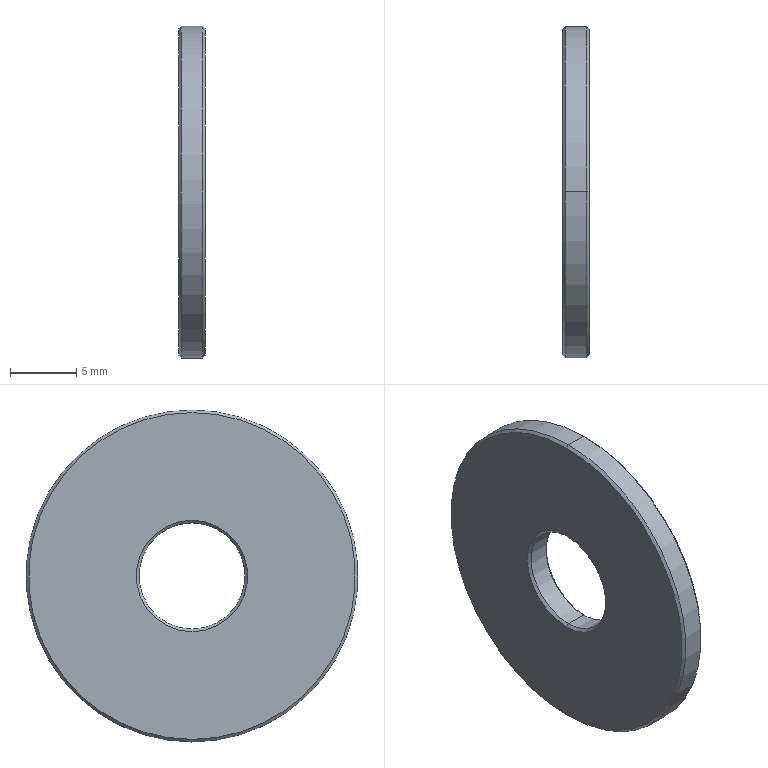Part | STEP file | WSSS25-8-2 | 1 solid | 14 faces | box 2 x 25 x 25 mm | volume 877.07 mm3 | cone 8 | cylinder 4 | plane 2 | commonest cylinder face diameters 8 x2 25 x2
STEP:
#1=CARTESIAN_POINT('',(2.,0.,-12.3));
#2=VERTEX_POINT('',#1);
#3=CARTESIAN_POINT('',(2.,0.,12.3));
#4=VERTEX_POINT('',#3);
#5=CARTESIAN_POINT('',(2.,0.,0.));
#6=DIRECTION('',(1.,0.,0.));
#7=DIRECTION('',(0.,0.,1.));
#8=AXIS2_PLACEMENT_3D('',#5,#6,#7);
#9=CIRCLE('',#8,12.3);
#10=EDGE_CURVE('',#2,#4,#9,.T.);
#11=ORIENTED_EDGE('',*,*,#10,.F.);
#12=CARTESIAN_POINT('',(1.8,0.,-12.5));
#13=VERTEX_POINT('',#12);
#14=CARTESIAN_POINT('',(1.8,0.,-12.5));
#15=DIRECTION('',(-0.7071,0.,-0.7071));
#16=VECTOR('',#15,1000.);
#17=LINE('',#14,#16);
#18=EDGE_CURVE('',#2,#13,#17,.T.);
#19=ORIENTED_EDGE('',*,*,#18,.T.);
#20=CARTESIAN_POINT('',(1.8,0.,12.5));
#21=VERTEX_POINT('',#20);
#22=CARTESIAN_POINT('',(1.8,0.,0.));
#23=DIRECTION('',(-1.,0.,0.));
#24=DIRECTION('',(0.,0.,1.));
#25=AXIS2_PLACEMENT_3D('',#22,#23,#24);
#26=CIRCLE('',#25,12.5);
#27=EDGE_CURVE('',#21,#13,#26,.T.);
#28=ORIENTED_EDGE('',*,*,#27,.F.);
#29=CARTESIAN_POINT('',(1.8,0.,12.5));
#30=DIRECTION('',(-0.7071,0.,0.7071));
#31=VECTOR('',#30,1000.);
#32=LINE('',#29,#31);
#33=EDGE_CURVE('',#4,#21,#32,.T.);
#34=ORIENTED_EDGE('',*,*,#33,.F.);
#35=EDGE_LOOP('',(#11,#19,#28,#34));
#36=FACE_OUTER_BOUND('',#35,.T.);
#37=CARTESIAN_POINT('',(1.8,0.,0.));
#38=DIRECTION('',(-1.,0.,0.));
#39=DIRECTION('',(0.,0.,1.));
#40=AXIS2_PLACEMENT_3D('',#37,#38,#39);
#41=CONICAL_SURFACE('',#40,12.5,0.7854);
#42=ADVANCED_FACE('',(#36),#41,.T.);
#43=CARTESIAN_POINT('',(1.8,0.,4.));
#44=VERTEX_POINT('',#43);
#45=CARTESIAN_POINT('',(1.8,0.,-4.));
#46=VERTEX_POINT('',#45);
#47=CARTESIAN_POINT('',(1.8,0.,0.));
#48=DIRECTION('',(1.,0.,0.));
#49=DIRECTION('',(0.,0.,1.));
#50=AXIS2_PLACEMENT_3D('',#47,#48,#49);
#51=CIRCLE('',#50,4.);
#52=EDGE_CURVE('',#44,#46,#51,.T.);
#53=ORIENTED_EDGE('',*,*,#52,.F.);
#54=CARTESIAN_POINT('',(2.,0.,4.2));
#55=VERTEX_POINT('',#54);
#56=CARTESIAN_POINT('',(2.,0.,4.2));
#57=DIRECTION('',(0.7071,0.,0.7071));
#58=VECTOR('',#57,1000.);
#59=LINE('',#56,#58);
#60=EDGE_CURVE('',#44,#55,#59,.T.);
#61=ORIENTED_EDGE('',*,*,#60,.T.);
#62=CARTESIAN_POINT('',(2.,0.,-4.2));
#63=VERTEX_POINT('',#62);
#64=CARTESIAN_POINT('',(2.,0.,0.));
#65=DIRECTION('',(-1.,0.,0.));
#66=DIRECTION('',(0.,0.,1.));
#67=AXIS2_PLACEMENT_3D('',#64,#65,#66);
#68=CIRCLE('',#67,4.2);
#69=EDGE_CURVE('',#63,#55,#68,.T.);
#70=ORIENTED_EDGE('',*,*,#69,.F.);
#71=CARTESIAN_POINT('',(2.,0.,-4.2));
#72=DIRECTION('',(0.7071,0.,-0.7071));
#73=VECTOR('',#72,1000.);
#74=LINE('',#71,#73);
#75=EDGE_CURVE('',#46,#63,#74,.T.);
#76=ORIENTED_EDGE('',*,*,#75,.F.);
#77=EDGE_LOOP('',(#53,#61,#70,#76));
#78=FACE_OUTER_BOUND('',#77,.T.);
#79=CARTESIAN_POINT('',(2.,0.,0.));
#80=DIRECTION('',(1.,0.,0.));
#81=DIRECTION('',(0.,0.,-1.));
#82=AXIS2_PLACEMENT_3D('',#79,#80,#81);
#83=CONICAL_SURFACE('',#82,4.2,0.7854);
#84=ADVANCED_FACE('',(#78),#83,.F.);
#85=CARTESIAN_POINT('',(0.,0.,12.3));
#86=VERTEX_POINT('',#85);
#87=CARTESIAN_POINT('',(0.,0.,-12.3));
#88=VERTEX_POINT('',#87);
#89=CARTESIAN_POINT('',(0.,0.,0.));
#90=DIRECTION('',(-1.,0.,0.));
#91=DIRECTION('',(0.,0.,-1.));
#92=AXIS2_PLACEMENT_3D('',#89,#90,#91);
#93=CIRCLE('',#92,12.3);
#94=EDGE_CURVE('',#86,#88,#93,.T.);
#95=ORIENTED_EDGE('',*,*,#94,.F.);
#96=CARTESIAN_POINT('',(0.2,0.,12.5));
#97=VERTEX_POINT('',#96);
#98=CARTESIAN_POINT('',(0.,0.,12.3));
#99=DIRECTION('',(0.7071,0.,0.7071));
#100=VECTOR('',#99,1000.);
#101=LINE('',#98,#100);
#102=EDGE_CURVE('',#86,#97,#101,.T.);
#103=ORIENTED_EDGE('',*,*,#102,.T.);
#104=CARTESIAN_POINT('',(0.2,0.,-12.5));
#105=VERTEX_POINT('',#104);
#106=CARTESIAN_POINT('',(0.2,0.,0.));
#107=DIRECTION('',(1.,0.,0.));
#108=DIRECTION('',(0.,0.,-1.));
#109=AXIS2_PLACEMENT_3D('',#106,#107,#108);
#110=CIRCLE('',#109,12.5);
#111=EDGE_CURVE('',#105,#97,#110,.T.);
#112=ORIENTED_EDGE('',*,*,#111,.F.);
#113=CARTESIAN_POINT('',(0.,0.,-12.3));
#114=DIRECTION('',(0.7071,0.,-0.7071));
#115=VECTOR('',#114,1000.);
#116=LINE('',#113,#115);
#117=EDGE_CURVE('',#88,#105,#116,.T.);
#118=ORIENTED_EDGE('',*,*,#117,.F.);
#119=EDGE_LOOP('',(#95,#103,#112,#118));
#120=FACE_OUTER_BOUND('',#119,.T.);
#121=CARTESIAN_POINT('',(0.,0.,0.));
#122=DIRECTION('',(1.,0.,0.));
#123=DIRECTION('',(0.,0.,-1.));
#124=AXIS2_PLACEMENT_3D('',#121,#122,#123);
#125=CONICAL_SURFACE('',#124,12.3,0.7854);
#126=ADVANCED_FACE('',(#120),#125,.T.);
#127=CARTESIAN_POINT('',(0.2,0.,-4.));
#128=VERTEX_POINT('',#127);
#129=CARTESIAN_POINT('',(0.2,0.,4.));
#130=VERTEX_POINT('',#129);
#131=CARTESIAN_POINT('',(0.2,0.,0.));
#132=DIRECTION('',(-1.,0.,0.));
#133=DIRECTION('',(0.,0.,-1.));
#134=AXIS2_PLACEMENT_3D('',#131,#132,#133);
#135=CIRCLE('',#134,4.);
#136=EDGE_CURVE('',#128,#130,#135,.T.);
#137=ORIENTED_EDGE('',*,*,#136,.F.);
#138=CARTESIAN_POINT('',(0.,0.,-4.2));
#139=VERTEX_POINT('',#138);
#140=CARTESIAN_POINT('',(0.2,0.,-4.));
#141=DIRECTION('',(-0.7071,0.,-0.7071));
#142=VECTOR('',#141,1000.);
#143=LINE('',#140,#142);
#144=EDGE_CURVE('',#128,#139,#143,.T.);
#145=ORIENTED_EDGE('',*,*,#144,.T.);
#146=CARTESIAN_POINT('',(0.,0.,4.2));
#147=VERTEX_POINT('',#146);
#148=CARTESIAN_POINT('',(0.,0.,0.));
#149=DIRECTION('',(1.,0.,0.));
#150=DIRECTION('',(0.,0.,-1.));
#151=AXIS2_PLACEMENT_3D('',#148,#149,#150);
#152=CIRCLE('',#151,4.2);
#153=EDGE_CURVE('',#147,#139,#152,.T.);
#154=ORIENTED_EDGE('',*,*,#153,.F.);
#155=CARTESIAN_POINT('',(0.2,0.,4.));
#156=DIRECTION('',(-0.7071,0.,0.7071));
#157=VECTOR('',#156,1000.);
#158=LINE('',#155,#157);
#159=EDGE_CURVE('',#130,#147,#158,.T.);
#160=ORIENTED_EDGE('',*,*,#159,.F.);
#161=EDGE_LOOP('',(#137,#145,#154,#160));
#162=FACE_OUTER_BOUND('',#161,.T.);
#163=CARTESIAN_POINT('',(0.2,0.,0.));
#164=DIRECTION('',(-1.,0.,0.));
#165=DIRECTION('',(0.,0.,1.));
#166=AXIS2_PLACEMENT_3D('',#163,#164,#165);
#167=CONICAL_SURFACE('',#166,4.,0.7854);
#168=ADVANCED_FACE('',(#162),#167,.F.);
#169=ORIENTED_EDGE('',*,*,#52,.T.);
#170=CARTESIAN_POINT('',(0.,0.,-4.));
#171=DIRECTION('',(-1.,0.,0.));
#172=VECTOR('',#171,1000.);
#173=LINE('',#170,#172);
#174=EDGE_CURVE('',#46,#128,#173,.T.);
#175=ORIENTED_EDGE('',*,*,#174,.T.);
#176=ORIENTED_EDGE('',*,*,#136,.T.);
#177=CARTESIAN_POINT('',(0.,0.,4.));
#178=DIRECTION('',(-1.,0.,0.));
#179=VECTOR('',#178,1000.);
#180=LINE('',#177,#179);
#181=EDGE_CURVE('',#44,#130,#180,.T.);
#182=ORIENTED_EDGE('',*,*,#181,.F.);
#183=EDGE_LOOP('',(#169,#175,#176,#182));
#184=FACE_OUTER_BOUND('',#183,.T.);
#185=CARTESIAN_POINT('',(0.,0.,0.));
#186=DIRECTION('',(-1.,0.,0.));
#187=DIRECTION('',(0.,0.,1.));
#188=AXIS2_PLACEMENT_3D('',#185,#186,#187);
#189=CYLINDRICAL_SURFACE('',#188,4.);
#190=ADVANCED_FACE('',(#184),#189,.F.);
#191=ORIENTED_EDGE('',*,*,#27,.T.);
#192=CARTESIAN_POINT('',(0.,0.,-12.5));
#193=DIRECTION('',(-1.,0.,0.));
#194=VECTOR('',#193,1000.);
#195=LINE('',#192,#194);
#196=EDGE_CURVE('',#13,#105,#195,.T.);
#197=ORIENTED_EDGE('',*,*,#196,.T.);
#198=ORIENTED_EDGE('',*,*,#111,.T.);
#199=CARTESIAN_POINT('',(0.,0.,12.5));
#200=DIRECTION('',(-1.,0.,0.));
#201=VECTOR('',#200,1000.);
#202=LINE('',#199,#201);
#203=EDGE_CURVE('',#21,#97,#202,.T.);
#204=ORIENTED_EDGE('',*,*,#203,.F.);
#205=EDGE_LOOP('',(#191,#197,#198,#204));
#206=FACE_OUTER_BOUND('',#205,.T.);
#207=CARTESIAN_POINT('',(0.,0.,0.));
#208=DIRECTION('',(-1.,0.,0.));
#209=DIRECTION('',(0.,0.,1.));
#210=AXIS2_PLACEMENT_3D('',#207,#208,#209);
#211=CYLINDRICAL_SURFACE('',#210,12.5);
#212=ADVANCED_FACE('',(#206),#211,.T.);
#213=ORIENTED_EDGE('',*,*,#153,.T.);
#214=CARTESIAN_POINT('',(0.,0.,0.));
#215=DIRECTION('',(1.,0.,0.));
#216=DIRECTION('',(0.,0.,-1.));
#217=AXIS2_PLACEMENT_3D('',#214,#215,#216);
#218=CIRCLE('',#217,4.2);
#219=EDGE_CURVE('',#139,#147,#218,.T.);
#220=ORIENTED_EDGE('',*,*,#219,.T.);
#221=EDGE_LOOP('',(#213,#220));
#222=FACE_BOUND('',#221,.T.);
#223=CARTESIAN_POINT('',(0.,0.,0.));
#224=DIRECTION('',(-1.,0.,0.));
#225=DIRECTION('',(0.,0.,-1.));
#226=AXIS2_PLACEMENT_3D('',#223,#224,#225);
#227=CIRCLE('',#226,12.3);
#228=EDGE_CURVE('',#88,#86,#227,.T.);
#229=ORIENTED_EDGE('',*,*,#228,.T.);
#230=ORIENTED_EDGE('',*,*,#94,.T.);
#231=EDGE_LOOP('',(#229,#230));
#232=FACE_OUTER_BOUND('',#231,.T.);
#233=CARTESIAN_POINT('',(0.,4.,0.));
#234=DIRECTION('',(1.,0.,0.));
#235=DIRECTION('',(0.,0.,-1.));
#236=AXIS2_PLACEMENT_3D('',#233,#234,#235);
#237=PLANE('',#236);
#238=ADVANCED_FACE('',(#222,#232),#237,.F.);
#239=ORIENTED_EDGE('',*,*,#196,.F.);
#240=CARTESIAN_POINT('',(1.8,0.,0.));
#241=DIRECTION('',(-1.,0.,0.));
#242=DIRECTION('',(0.,0.,1.));
#243=AXIS2_PLACEMENT_3D('',#240,#241,#242);
#244=CIRCLE('',#243,12.5);
#245=EDGE_CURVE('',#13,#21,#244,.T.);
#246=ORIENTED_EDGE('',*,*,#245,.T.);
#247=ORIENTED_EDGE('',*,*,#203,.T.);
#248=CARTESIAN_POINT('',(0.2,0.,0.));
#249=DIRECTION('',(1.,0.,0.));
#250=DIRECTION('',(0.,0.,-1.));
#251=AXIS2_PLACEMENT_3D('',#248,#249,#250);
#252=CIRCLE('',#251,12.5);
#253=EDGE_CURVE('',#97,#105,#252,.T.);
#254=ORIENTED_EDGE('',*,*,#253,.T.);
#255=EDGE_LOOP('',(#239,#246,#247,#254));
#256=FACE_OUTER_BOUND('',#255,.T.);
#257=CARTESIAN_POINT('',(0.,0.,0.));
#258=DIRECTION('',(-1.,0.,0.));
#259=DIRECTION('',(0.,0.,1.));
#260=AXIS2_PLACEMENT_3D('',#257,#258,#259);
#261=CYLINDRICAL_SURFACE('',#260,12.5);
#262=ADVANCED_FACE('',(#256),#261,.T.);
#263=ORIENTED_EDGE('',*,*,#69,.T.);
#264=CARTESIAN_POINT('',(2.,0.,0.));
#265=DIRECTION('',(-1.,0.,0.));
#266=DIRECTION('',(0.,0.,1.));
#267=AXIS2_PLACEMENT_3D('',#264,#265,#266);
#268=CIRCLE('',#267,4.2);
#269=EDGE_CURVE('',#55,#63,#268,.T.);
#270=ORIENTED_EDGE('',*,*,#269,.T.);
#271=EDGE_LOOP('',(#263,#270));
#272=FACE_BOUND('',#271,.T.);
#273=CARTESIAN_POINT('',(2.,0.,0.));
#274=DIRECTION('',(1.,0.,0.));
#275=DIRECTION('',(0.,0.,1.));
#276=AXIS2_PLACEMENT_3D('',#273,#274,#275);
#277=CIRCLE('',#276,12.3);
#278=EDGE_CURVE('',#4,#2,#277,.T.);
#279=ORIENTED_EDGE('',*,*,#278,.T.);
#280=ORIENTED_EDGE('',*,*,#10,.T.);
#281=EDGE_LOOP('',(#279,#280));
#282=FACE_OUTER_BOUND('',#281,.T.);
#283=CARTESIAN_POINT('',(2.,4.,0.));
#284=DIRECTION('',(-1.,0.,0.));
#285=DIRECTION('',(0.,0.,1.));
#286=AXIS2_PLACEMENT_3D('',#283,#284,#285);
#287=PLANE('',#286);
#288=ADVANCED_FACE('',(#272,#282),#287,.F.);
#289=ORIENTED_EDGE('',*,*,#174,.F.);
#290=CARTESIAN_POINT('',(1.8,0.,0.));
#291=DIRECTION('',(1.,0.,0.));
#292=DIRECTION('',(0.,0.,1.));
#293=AXIS2_PLACEMENT_3D('',#290,#291,#292);
#294=CIRCLE('',#293,4.);
#295=EDGE_CURVE('',#46,#44,#294,.T.);
#296=ORIENTED_EDGE('',*,*,#295,.T.);
#297=ORIENTED_EDGE('',*,*,#181,.T.);
#298=CARTESIAN_POINT('',(0.2,0.,0.));
#299=DIRECTION('',(-1.,0.,0.));
#300=DIRECTION('',(0.,0.,-1.));
#301=AXIS2_PLACEMENT_3D('',#298,#299,#300);
#302=CIRCLE('',#301,4.);
#303=EDGE_CURVE('',#130,#128,#302,.T.);
#304=ORIENTED_EDGE('',*,*,#303,.T.);
#305=EDGE_LOOP('',(#289,#296,#297,#304));
#306=FACE_OUTER_BOUND('',#305,.T.);
#307=CARTESIAN_POINT('',(0.,0.,0.));
#308=DIRECTION('',(-1.,0.,0.));
#309=DIRECTION('',(0.,0.,1.));
#310=AXIS2_PLACEMENT_3D('',#307,#308,#309);
#311=CYLINDRICAL_SURFACE('',#310,4.);
#312=ADVANCED_FACE('',(#306),#311,.F.);
#313=ORIENTED_EDGE('',*,*,#144,.F.);
#314=ORIENTED_EDGE('',*,*,#303,.F.);
#315=ORIENTED_EDGE('',*,*,#159,.T.);
#316=ORIENTED_EDGE('',*,*,#219,.F.);
#317=EDGE_LOOP('',(#313,#314,#315,#316));
#318=FACE_OUTER_BOUND('',#317,.T.);
#319=CARTESIAN_POINT('',(0.2,0.,0.));
#320=DIRECTION('',(-1.,0.,0.));
#321=DIRECTION('',(0.,0.,1.));
#322=AXIS2_PLACEMENT_3D('',#319,#320,#321);
#323=CONICAL_SURFACE('',#322,4.,0.7854);
#324=ADVANCED_FACE('',(#318),#323,.F.);
#325=ORIENTED_EDGE('',*,*,#102,.F.);
#326=ORIENTED_EDGE('',*,*,#228,.F.);
#327=ORIENTED_EDGE('',*,*,#117,.T.);
#328=ORIENTED_EDGE('',*,*,#253,.F.);
#329=EDGE_LOOP('',(#325,#326,#327,#328));
#330=FACE_OUTER_BOUND('',#329,.T.);
#331=CARTESIAN_POINT('',(0.,0.,0.));
#332=DIRECTION('',(1.,0.,0.));
#333=DIRECTION('',(0.,0.,-1.));
#334=AXIS2_PLACEMENT_3D('',#331,#332,#333);
#335=CONICAL_SURFACE('',#334,12.3,0.7854);
#336=ADVANCED_FACE('',(#330),#335,.T.);
#337=ORIENTED_EDGE('',*,*,#60,.F.);
#338=ORIENTED_EDGE('',*,*,#295,.F.);
#339=ORIENTED_EDGE('',*,*,#75,.T.);
#340=ORIENTED_EDGE('',*,*,#269,.F.);
#341=EDGE_LOOP('',(#337,#338,#339,#340));
#342=FACE_OUTER_BOUND('',#341,.T.);
#343=CARTESIAN_POINT('',(2.,0.,0.));
#344=DIRECTION('',(1.,0.,0.));
#345=DIRECTION('',(0.,0.,-1.));
#346=AXIS2_PLACEMENT_3D('',#343,#344,#345);
#347=CONICAL_SURFACE('',#346,4.2,0.7854);
#348=ADVANCED_FACE('',(#342),#347,.F.);
#349=ORIENTED_EDGE('',*,*,#18,.F.);
#350=ORIENTED_EDGE('',*,*,#278,.F.);
#351=ORIENTED_EDGE('',*,*,#33,.T.);
#352=ORIENTED_EDGE('',*,*,#245,.F.);
#353=EDGE_LOOP('',(#349,#350,#351,#352));
#354=FACE_OUTER_BOUND('',#353,.T.);
#355=CARTESIAN_POINT('',(1.8,0.,0.));
#356=DIRECTION('',(-1.,0.,0.));
#357=DIRECTION('',(0.,0.,1.));
#358=AXIS2_PLACEMENT_3D('',#355,#356,#357);
#359=CONICAL_SURFACE('',#358,12.5,0.7854);
#360=ADVANCED_FACE('',(#354),#359,.T.);
#361=CLOSED_SHELL('',(#42,#84,#126,#168,#190,#212,#238,#262,#288,#312,#324,#336,#348,#360));
#362=MANIFOLD_SOLID_BREP('',#361);
#363=CARTESIAN_POINT('',(0.,0.,0.));
#364=DIRECTION('',(0.,0.,1.));
#365=DIRECTION('',(1.,0.,0.));
#366=AXIS2_PLACEMENT_3D('',#363,#364,#365);
#367=(LENGTH_UNIT()NAMED_UNIT(*)SI_UNIT(.MILLI.,.METRE.));
#368=UNCERTAINTY_MEASURE_WITH_UNIT(LENGTH_MEASURE(0.00001),#367,'','');
#369=(NAMED_UNIT(*)PLANE_ANGLE_UNIT()SI_UNIT($,.RADIAN.));
#370=(NAMED_UNIT(*)SI_UNIT($,.STERADIAN.)SOLID_ANGLE_UNIT());
#371=(GEOMETRIC_REPRESENTATION_CONTEXT(3)GLOBAL_UNCERTAINTY_ASSIGNED_CONTEXT((#368))GLOBAL_UNIT_ASSIGNED_CONTEXT((#367,#369,#370))REPRESENTATION_CONTEXT('',''));
#372=ADVANCED_BREP_SHAPE_REPRESENTATION('',(#362,#366),#371);